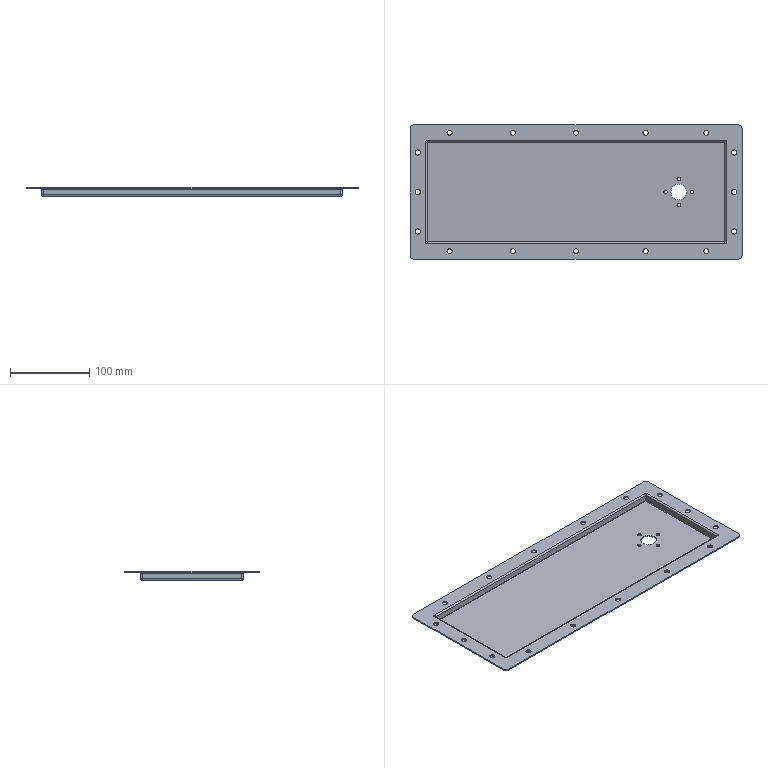Part | NX | features BREP 1 | 1 solid | 103 faces | box 420 x 170 x 11.5 mm | volume 119203 mm3 | cylinder 70 | plane 16 | sphere 9 | torus 8 | commonest cylinder face diameters 6.5 x32 1 x12 4 x12 4.5 x8 10 x4 20 x2